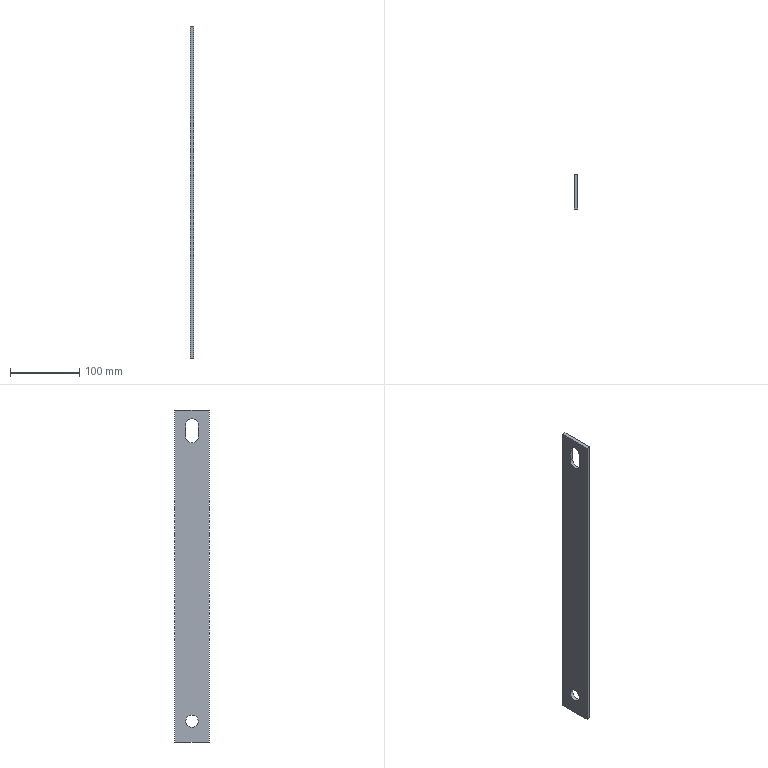Part | NX | features solid 2 | 1 solid | 11 faces | box 5 x 50 x 480 mm | volume 115925 mm3 | plane 8 | cylinder 3 | commonest cylinder face diameters 18 x3
STEP:
#1=CARTESIAN_POINT('',(-1270.,-535.,-215.));
#2=VERTEX_POINT('',#1);
#3=CARTESIAN_POINT('',(-1270.,-535.,265.));
#4=VERTEX_POINT('',#3);
#5=CARTESIAN_POINT('',(-1270.,-535.,-125.));
#6=DIRECTION('',(0.,0.,1.));
#7=VECTOR('',#6,1000.);
#8=LINE('',#5,#7);
#9=EDGE_CURVE('',#2,#4,#8,.T.);
#10=ORIENTED_EDGE('',*,*,#9,.F.);
#11=CARTESIAN_POINT('',(-1270.,-485.,-215.));
#12=VERTEX_POINT('',#11);
#13=CARTESIAN_POINT('',(-1270.,-510.,-215.));
#14=DIRECTION('',(0.,1.,0.));
#15=VECTOR('',#14,1000.);
#16=LINE('',#13,#15);
#17=EDGE_CURVE('',#2,#12,#16,.T.);
#18=ORIENTED_EDGE('',*,*,#17,.T.);
#19=CARTESIAN_POINT('',(-1270.,-485.,265.));
#20=VERTEX_POINT('',#19);
#21=CARTESIAN_POINT('',(-1270.,-485.,-125.));
#22=DIRECTION('',(0.,0.,1.));
#23=VECTOR('',#22,1000.);
#24=LINE('',#21,#23);
#25=EDGE_CURVE('',#12,#20,#24,.T.);
#26=ORIENTED_EDGE('',*,*,#25,.T.);
#27=CARTESIAN_POINT('',(-1270.,-510.,265.));
#28=DIRECTION('',(0.,-1.,0.));
#29=VECTOR('',#28,1000.);
#30=LINE('',#27,#29);
#31=EDGE_CURVE('',#20,#4,#30,.T.);
#32=ORIENTED_EDGE('',*,*,#31,.T.);
#33=EDGE_LOOP('',(#10,#18,#26,#32));
#34=FACE_BOUND('',#33,.T.);
#35=CARTESIAN_POINT('',(-1270.,-510.,-176.));
#36=VERTEX_POINT('',#35);
#37=CARTESIAN_POINT('',(-1270.,-510.,-185.));
#38=DIRECTION('',(-1.,0.,0.));
#39=DIRECTION('',(0.,0.,1.));
#40=AXIS2_PLACEMENT_3D('',#37,#38,#39);
#41=CIRCLE('',#40,9.);
#42=EDGE_CURVE('',#36,#36,#41,.T.);
#43=ORIENTED_EDGE('',*,*,#42,.T.);
#44=EDGE_LOOP('',(#43));
#45=FACE_BOUND('',#44,.T.);
#46=CARTESIAN_POINT('',(-1270.,-519.,226.5));
#47=VERTEX_POINT('',#46);
#48=CARTESIAN_POINT('',(-1270.,-519.,243.5));
#49=VERTEX_POINT('',#48);
#50=CARTESIAN_POINT('',(-1270.,-519.,226.5));
#51=DIRECTION('',(0.,0.,1.));
#52=VECTOR('',#51,1000.);
#53=LINE('',#50,#52);
#54=EDGE_CURVE('',#47,#49,#53,.T.);
#55=ORIENTED_EDGE('',*,*,#54,.T.);
#56=CARTESIAN_POINT('',(-1270.,-501.,243.5));
#57=VERTEX_POINT('',#56);
#58=CARTESIAN_POINT('',(-1270.,-510.,243.5));
#59=DIRECTION('',(-1.,0.,0.));
#60=DIRECTION('',(0.,0.,1.));
#61=AXIS2_PLACEMENT_3D('',#58,#59,#60);
#62=CIRCLE('',#61,9.);
#63=EDGE_CURVE('',#49,#57,#62,.T.);
#64=ORIENTED_EDGE('',*,*,#63,.T.);
#65=CARTESIAN_POINT('',(-1270.,-501.,226.5));
#66=VERTEX_POINT('',#65);
#67=CARTESIAN_POINT('',(-1270.,-501.,226.5));
#68=DIRECTION('',(0.,0.,1.));
#69=VECTOR('',#68,1000.);
#70=LINE('',#67,#69);
#71=EDGE_CURVE('',#66,#57,#70,.T.);
#72=ORIENTED_EDGE('',*,*,#71,.F.);
#73=CARTESIAN_POINT('',(-1270.,-510.,226.5));
#74=DIRECTION('',(-1.,0.,0.));
#75=DIRECTION('',(0.,0.,1.));
#76=AXIS2_PLACEMENT_3D('',#73,#74,#75);
#77=CIRCLE('',#76,9.);
#78=EDGE_CURVE('',#66,#47,#77,.T.);
#79=ORIENTED_EDGE('',*,*,#78,.T.);
#80=EDGE_LOOP('',(#55,#64,#72,#79));
#81=FACE_BOUND('',#80,.T.);
#82=CARTESIAN_POINT('',(-1270.,-510.,-125.));
#83=DIRECTION('',(1.,0.,0.));
#84=DIRECTION('',(0.,0.,-1.));
#85=AXIS2_PLACEMENT_3D('',#82,#83,#84);
#86=PLANE('',#85);
#87=ADVANCED_FACE('',(#34,#45,#81),#86,.T.);
#88=ORIENTED_EDGE('',*,*,#25,.F.);
#89=CARTESIAN_POINT('',(-1275.,-485.,-215.));
#90=VERTEX_POINT('',#89);
#91=CARTESIAN_POINT('',(-1272.5,-485.,-215.));
#92=DIRECTION('',(-1.,0.,0.));
#93=VECTOR('',#92,1000.);
#94=LINE('',#91,#93);
#95=EDGE_CURVE('',#12,#90,#94,.T.);
#96=ORIENTED_EDGE('',*,*,#95,.T.);
#97=CARTESIAN_POINT('',(-1275.,-485.,265.));
#98=VERTEX_POINT('',#97);
#99=CARTESIAN_POINT('',(-1275.,-485.,-125.));
#100=DIRECTION('',(0.,0.,1.));
#101=VECTOR('',#100,1000.);
#102=LINE('',#99,#101);
#103=EDGE_CURVE('',#90,#98,#102,.T.);
#104=ORIENTED_EDGE('',*,*,#103,.T.);
#105=CARTESIAN_POINT('',(-1272.5,-485.,265.));
#106=DIRECTION('',(1.,0.,0.));
#107=VECTOR('',#106,1000.);
#108=LINE('',#105,#107);
#109=EDGE_CURVE('',#98,#20,#108,.T.);
#110=ORIENTED_EDGE('',*,*,#109,.T.);
#111=EDGE_LOOP('',(#88,#96,#104,#110));
#112=FACE_BOUND('',#111,.T.);
#113=CARTESIAN_POINT('',(-1272.5,-485.,-125.));
#114=DIRECTION('',(0.,1.,0.));
#115=DIRECTION('',(0.,0.,1.));
#116=AXIS2_PLACEMENT_3D('',#113,#114,#115);
#117=PLANE('',#116);
#118=ADVANCED_FACE('',(#112),#117,.T.);
#119=ORIENTED_EDGE('',*,*,#103,.F.);
#120=CARTESIAN_POINT('',(-1275.,-535.,-215.));
#121=VERTEX_POINT('',#120);
#122=CARTESIAN_POINT('',(-1275.,-510.,-215.));
#123=DIRECTION('',(0.,-1.,0.));
#124=VECTOR('',#123,1000.);
#125=LINE('',#122,#124);
#126=EDGE_CURVE('',#90,#121,#125,.T.);
#127=ORIENTED_EDGE('',*,*,#126,.T.);
#128=CARTESIAN_POINT('',(-1275.,-535.,265.));
#129=VERTEX_POINT('',#128);
#130=CARTESIAN_POINT('',(-1275.,-535.,-125.));
#131=DIRECTION('',(0.,0.,1.));
#132=VECTOR('',#131,1000.);
#133=LINE('',#130,#132);
#134=EDGE_CURVE('',#121,#129,#133,.T.);
#135=ORIENTED_EDGE('',*,*,#134,.T.);
#136=CARTESIAN_POINT('',(-1275.,-510.,265.));
#137=DIRECTION('',(0.,1.,0.));
#138=VECTOR('',#137,1000.);
#139=LINE('',#136,#138);
#140=EDGE_CURVE('',#129,#98,#139,.T.);
#141=ORIENTED_EDGE('',*,*,#140,.T.);
#142=EDGE_LOOP('',(#119,#127,#135,#141));
#143=FACE_BOUND('',#142,.T.);
#144=CARTESIAN_POINT('',(-1275.,-510.,-194.));
#145=VERTEX_POINT('',#144);
#146=CARTESIAN_POINT('',(-1275.,-510.,-185.));
#147=DIRECTION('',(1.,0.,0.));
#148=DIRECTION('',(0.,0.,-1.));
#149=AXIS2_PLACEMENT_3D('',#146,#147,#148);
#150=CIRCLE('',#149,9.);
#151=EDGE_CURVE('',#145,#145,#150,.T.);
#152=ORIENTED_EDGE('',*,*,#151,.T.);
#153=EDGE_LOOP('',(#152));
#154=FACE_BOUND('',#153,.T.);
#155=CARTESIAN_POINT('',(-1275.,-519.,226.5));
#156=VERTEX_POINT('',#155);
#157=CARTESIAN_POINT('',(-1275.,-519.,243.5));
#158=VERTEX_POINT('',#157);
#159=CARTESIAN_POINT('',(-1275.,-519.,226.5));
#160=DIRECTION('',(0.,0.,1.));
#161=VECTOR('',#160,1000.);
#162=LINE('',#159,#161);
#163=EDGE_CURVE('',#156,#158,#162,.T.);
#164=ORIENTED_EDGE('',*,*,#163,.F.);
#165=CARTESIAN_POINT('',(-1275.,-501.,226.5));
#166=VERTEX_POINT('',#165);
#167=CARTESIAN_POINT('',(-1275.,-510.,226.5));
#168=DIRECTION('',(1.,0.,0.));
#169=DIRECTION('',(0.,0.,-1.));
#170=AXIS2_PLACEMENT_3D('',#167,#168,#169);
#171=CIRCLE('',#170,9.);
#172=EDGE_CURVE('',#156,#166,#171,.T.);
#173=ORIENTED_EDGE('',*,*,#172,.T.);
#174=CARTESIAN_POINT('',(-1275.,-501.,243.5));
#175=VERTEX_POINT('',#174);
#176=CARTESIAN_POINT('',(-1275.,-501.,226.5));
#177=DIRECTION('',(0.,0.,1.));
#178=VECTOR('',#177,1000.);
#179=LINE('',#176,#178);
#180=EDGE_CURVE('',#166,#175,#179,.T.);
#181=ORIENTED_EDGE('',*,*,#180,.T.);
#182=CARTESIAN_POINT('',(-1275.,-510.,243.5));
#183=DIRECTION('',(1.,0.,0.));
#184=DIRECTION('',(0.,0.,-1.));
#185=AXIS2_PLACEMENT_3D('',#182,#183,#184);
#186=CIRCLE('',#185,9.);
#187=EDGE_CURVE('',#175,#158,#186,.T.);
#188=ORIENTED_EDGE('',*,*,#187,.T.);
#189=EDGE_LOOP('',(#164,#173,#181,#188));
#190=FACE_BOUND('',#189,.T.);
#191=CARTESIAN_POINT('',(-1275.,-510.,-125.));
#192=DIRECTION('',(-1.,0.,0.));
#193=DIRECTION('',(0.,0.,1.));
#194=AXIS2_PLACEMENT_3D('',#191,#192,#193);
#195=PLANE('',#194);
#196=ADVANCED_FACE('',(#143,#154,#190),#195,.T.);
#197=ORIENTED_EDGE('',*,*,#134,.F.);
#198=CARTESIAN_POINT('',(-1272.5,-535.,-215.));
#199=DIRECTION('',(1.,0.,0.));
#200=VECTOR('',#199,1000.);
#201=LINE('',#198,#200);
#202=EDGE_CURVE('',#121,#2,#201,.T.);
#203=ORIENTED_EDGE('',*,*,#202,.T.);
#204=ORIENTED_EDGE('',*,*,#9,.T.);
#205=CARTESIAN_POINT('',(-1272.5,-535.,265.));
#206=DIRECTION('',(-1.,0.,0.));
#207=VECTOR('',#206,1000.);
#208=LINE('',#205,#207);
#209=EDGE_CURVE('',#4,#129,#208,.T.);
#210=ORIENTED_EDGE('',*,*,#209,.T.);
#211=EDGE_LOOP('',(#197,#203,#204,#210));
#212=FACE_BOUND('',#211,.T.);
#213=CARTESIAN_POINT('',(-1272.5,-535.,-125.));
#214=DIRECTION('',(0.,-1.,0.));
#215=DIRECTION('',(0.,0.,-1.));
#216=AXIS2_PLACEMENT_3D('',#213,#214,#215);
#217=PLANE('',#216);
#218=ADVANCED_FACE('',(#212),#217,.T.);
#219=ORIENTED_EDGE('',*,*,#17,.F.);
#220=ORIENTED_EDGE('',*,*,#202,.F.);
#221=ORIENTED_EDGE('',*,*,#126,.F.);
#222=ORIENTED_EDGE('',*,*,#95,.F.);
#223=EDGE_LOOP('',(#219,#220,#221,#222));
#224=FACE_BOUND('',#223,.T.);
#225=CARTESIAN_POINT('',(-1272.5,-510.,-215.));
#226=DIRECTION('',(0.,0.,-1.));
#227=DIRECTION('',(-1.,0.,0.));
#228=AXIS2_PLACEMENT_3D('',#225,#226,#227);
#229=PLANE('',#228);
#230=ADVANCED_FACE('',(#224),#229,.T.);
#231=ORIENTED_EDGE('',*,*,#151,.F.);
#232=EDGE_LOOP('',(#231));
#233=FACE_BOUND('',#232,.T.);
#234=ORIENTED_EDGE('',*,*,#42,.F.);
#235=EDGE_LOOP('',(#234));
#236=FACE_BOUND('',#235,.T.);
#237=CARTESIAN_POINT('',(-1270.,-510.,-185.));
#238=DIRECTION('',(-1.,0.,0.));
#239=DIRECTION('',(0.,0.,1.));
#240=AXIS2_PLACEMENT_3D('',#237,#238,#239);
#241=CYLINDRICAL_SURFACE('',#240,9.);
#242=ADVANCED_FACE('',(#233,#236),#241,.F.);
#243=ORIENTED_EDGE('',*,*,#172,.F.);
#244=CARTESIAN_POINT('',(-1272.5,-519.,226.5));
#245=DIRECTION('',(1.,0.,0.));
#246=VECTOR('',#245,1000.);
#247=LINE('',#244,#246);
#248=EDGE_CURVE('',#156,#47,#247,.T.);
#249=ORIENTED_EDGE('',*,*,#248,.T.);
#250=ORIENTED_EDGE('',*,*,#78,.F.);
#251=CARTESIAN_POINT('',(-1272.5,-501.,226.5));
#252=DIRECTION('',(-1.,0.,0.));
#253=VECTOR('',#252,1000.);
#254=LINE('',#251,#253);
#255=EDGE_CURVE('',#66,#166,#254,.T.);
#256=ORIENTED_EDGE('',*,*,#255,.T.);
#257=EDGE_LOOP('',(#243,#249,#250,#256));
#258=FACE_BOUND('',#257,.T.);
#259=CARTESIAN_POINT('',(-1270.,-510.,226.5));
#260=DIRECTION('',(-1.,0.,0.));
#261=DIRECTION('',(0.,0.,1.));
#262=AXIS2_PLACEMENT_3D('',#259,#260,#261);
#263=CYLINDRICAL_SURFACE('',#262,9.);
#264=ADVANCED_FACE('',(#258),#263,.F.);
#265=ORIENTED_EDGE('',*,*,#180,.F.);
#266=ORIENTED_EDGE('',*,*,#255,.F.);
#267=ORIENTED_EDGE('',*,*,#71,.T.);
#268=CARTESIAN_POINT('',(-1272.5,-501.,243.5));
#269=DIRECTION('',(1.,0.,0.));
#270=VECTOR('',#269,1000.);
#271=LINE('',#268,#270);
#272=EDGE_CURVE('',#175,#57,#271,.T.);
#273=ORIENTED_EDGE('',*,*,#272,.F.);
#274=EDGE_LOOP('',(#265,#266,#267,#273));
#275=FACE_BOUND('',#274,.T.);
#276=CARTESIAN_POINT('',(-1272.5,-501.,226.5));
#277=DIRECTION('',(0.,1.,0.));
#278=DIRECTION('',(0.,0.,1.));
#279=AXIS2_PLACEMENT_3D('',#276,#277,#278);
#280=PLANE('',#279);
#281=ADVANCED_FACE('',(#275),#280,.F.);
#282=CARTESIAN_POINT('',(-1272.5,-519.,243.5));
#283=DIRECTION('',(-1.,0.,0.));
#284=VECTOR('',#283,1000.);
#285=LINE('',#282,#284);
#286=EDGE_CURVE('',#49,#158,#285,.T.);
#287=ORIENTED_EDGE('',*,*,#286,.T.);
#288=ORIENTED_EDGE('',*,*,#187,.F.);
#289=ORIENTED_EDGE('',*,*,#272,.T.);
#290=ORIENTED_EDGE('',*,*,#63,.F.);
#291=EDGE_LOOP('',(#287,#288,#289,#290));
#292=FACE_BOUND('',#291,.T.);
#293=CARTESIAN_POINT('',(-1270.,-510.,243.5));
#294=DIRECTION('',(-1.,0.,0.));
#295=DIRECTION('',(0.,0.,1.));
#296=AXIS2_PLACEMENT_3D('',#293,#294,#295);
#297=CYLINDRICAL_SURFACE('',#296,9.);
#298=ADVANCED_FACE('',(#292),#297,.F.);
#299=ORIENTED_EDGE('',*,*,#54,.F.);
#300=ORIENTED_EDGE('',*,*,#248,.F.);
#301=ORIENTED_EDGE('',*,*,#163,.T.);
#302=ORIENTED_EDGE('',*,*,#286,.F.);
#303=EDGE_LOOP('',(#299,#300,#301,#302));
#304=FACE_BOUND('',#303,.T.);
#305=CARTESIAN_POINT('',(-1272.5,-519.,226.5));
#306=DIRECTION('',(0.,-1.,0.));
#307=DIRECTION('',(0.,0.,-1.));
#308=AXIS2_PLACEMENT_3D('',#305,#306,#307);
#309=PLANE('',#308);
#310=ADVANCED_FACE('',(#304),#309,.F.);
#311=ORIENTED_EDGE('',*,*,#209,.F.);
#312=ORIENTED_EDGE('',*,*,#31,.F.);
#313=ORIENTED_EDGE('',*,*,#109,.F.);
#314=ORIENTED_EDGE('',*,*,#140,.F.);
#315=EDGE_LOOP('',(#311,#312,#313,#314));
#316=FACE_BOUND('',#315,.T.);
#317=CARTESIAN_POINT('',(-1272.5,-510.,265.));
#318=DIRECTION('',(0.,0.,1.));
#319=DIRECTION('',(1.,0.,0.));
#320=AXIS2_PLACEMENT_3D('',#317,#318,#319);
#321=PLANE('',#320);
#322=ADVANCED_FACE('',(#316),#321,.T.);
#323=CLOSED_SHELL('',(#87,#118,#196,#218,#230,#242,#264,#281,#298,#310,#322));
#324=MANIFOLD_SOLID_BREP('',#323);
#325=(LENGTH_UNIT()NAMED_UNIT(*)SI_UNIT(.MILLI.,.METRE.));
#326=UNCERTAINTY_MEASURE_WITH_UNIT(LENGTH_MEASURE(0.00001),#325,'','');
#327=(NAMED_UNIT(*)PLANE_ANGLE_UNIT()SI_UNIT($,.RADIAN.));
#328=(NAMED_UNIT(*)SI_UNIT($,.STERADIAN.)SOLID_ANGLE_UNIT());
#329=(GEOMETRIC_REPRESENTATION_CONTEXT(3)GLOBAL_UNCERTAINTY_ASSIGNED_CONTEXT((#326))GLOBAL_UNIT_ASSIGNED_CONTEXT((#325,#327,#328))REPRESENTATION_CONTEXT('',''));
#330=ADVANCED_BREP_SHAPE_REPRESENTATION('',(#324),#329);